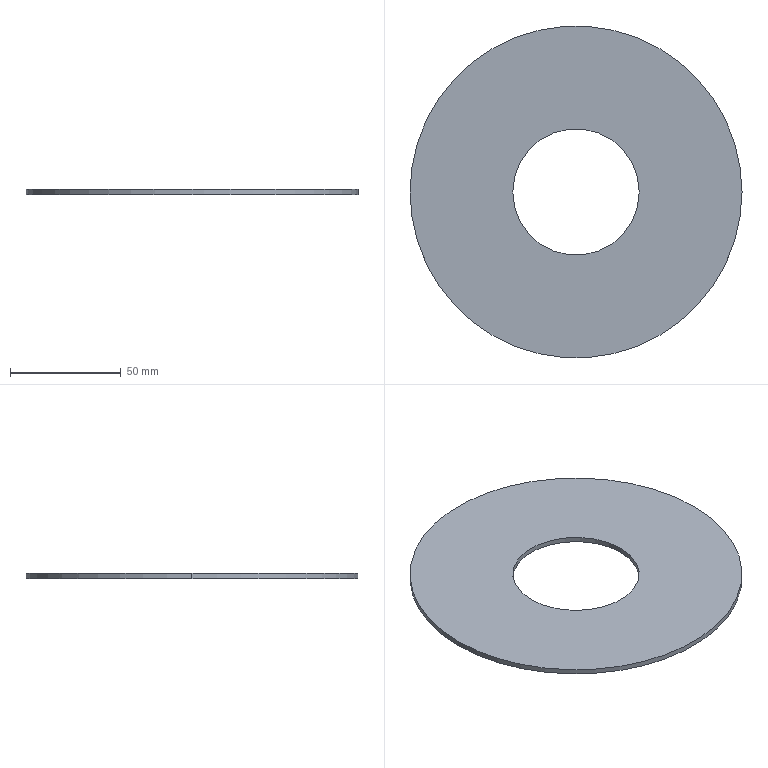Part | SolidWorks | features FlatPattern 1, SMBaseFlange 1, SheetMetal 1 | 1 solid | 6 faces | box 150 x 150 x 2.3 mm | volume 34755 mm3 | cylinder 4 | plane 2 | commonest cylinder face diameters 57.1 x2 150 x2
STEP:
#1=CARTESIAN_POINT('',(-28.55,0.,-2.3));
#2=VERTEX_POINT('',#1);
#3=CARTESIAN_POINT('',(28.55,0.,-2.3));
#4=VERTEX_POINT('',#3);
#5=CARTESIAN_POINT('',(0.,0.,-2.3));
#6=DIRECTION('',(0.,0.,1.));
#7=DIRECTION('',(1.,0.,0.));
#8=AXIS2_PLACEMENT_3D('',#5,#6,#7);
#9=CIRCLE('',#8,28.55);
#10=EDGE_CURVE('',#2,#4,#9,.T.);
#11=ORIENTED_EDGE('',*,*,#10,.F.);
#12=CARTESIAN_POINT('',(-28.55,0.,0.));
#13=VERTEX_POINT('',#12);
#14=CARTESIAN_POINT('',(-28.55,0.,-2.3));
#15=DIRECTION('',(0.,0.,1.));
#16=VECTOR('',#15,1000.);
#17=LINE('',#14,#16);
#18=EDGE_CURVE('',#2,#13,#17,.T.);
#19=ORIENTED_EDGE('',*,*,#18,.T.);
#20=CARTESIAN_POINT('',(28.55,0.,0.));
#21=VERTEX_POINT('',#20);
#22=CARTESIAN_POINT('',(0.,0.,0.));
#23=DIRECTION('',(0.,0.,1.));
#24=DIRECTION('',(1.,0.,0.));
#25=AXIS2_PLACEMENT_3D('',#22,#23,#24);
#26=CIRCLE('',#25,28.55);
#27=EDGE_CURVE('',#13,#21,#26,.T.);
#28=ORIENTED_EDGE('',*,*,#27,.T.);
#29=CARTESIAN_POINT('',(28.55,0.,-2.3));
#30=DIRECTION('',(0.,0.,1.));
#31=VECTOR('',#30,1000.);
#32=LINE('',#29,#31);
#33=EDGE_CURVE('',#4,#21,#32,.T.);
#34=ORIENTED_EDGE('',*,*,#33,.F.);
#35=EDGE_LOOP('',(#11,#19,#28,#34));
#36=FACE_OUTER_BOUND('',#35,.T.);
#37=CARTESIAN_POINT('',(0.,0.,-2.3));
#38=DIRECTION('',(0.,0.,1.));
#39=DIRECTION('',(1.,0.,0.));
#40=AXIS2_PLACEMENT_3D('',#37,#38,#39);
#41=CYLINDRICAL_SURFACE('',#40,28.55);
#42=ADVANCED_FACE('',(#36),#41,.F.);
#43=CARTESIAN_POINT('',(75.,0.,-2.3));
#44=VERTEX_POINT('',#43);
#45=CARTESIAN_POINT('',(-75.,0.,-2.3));
#46=VERTEX_POINT('',#45);
#47=CARTESIAN_POINT('',(0.,0.,-2.3));
#48=DIRECTION('',(0.,0.,1.));
#49=DIRECTION('',(1.,0.,0.));
#50=AXIS2_PLACEMENT_3D('',#47,#48,#49);
#51=CIRCLE('',#50,75.);
#52=EDGE_CURVE('',#44,#46,#51,.T.);
#53=ORIENTED_EDGE('',*,*,#52,.T.);
#54=CARTESIAN_POINT('',(-75.,0.,0.));
#55=VERTEX_POINT('',#54);
#56=CARTESIAN_POINT('',(-75.,0.,-2.3));
#57=DIRECTION('',(0.,0.,1.));
#58=VECTOR('',#57,1000.);
#59=LINE('',#56,#58);
#60=EDGE_CURVE('',#46,#55,#59,.T.);
#61=ORIENTED_EDGE('',*,*,#60,.T.);
#62=CARTESIAN_POINT('',(75.,0.,0.));
#63=VERTEX_POINT('',#62);
#64=CARTESIAN_POINT('',(0.,0.,0.));
#65=DIRECTION('',(0.,0.,1.));
#66=DIRECTION('',(1.,0.,0.));
#67=AXIS2_PLACEMENT_3D('',#64,#65,#66);
#68=CIRCLE('',#67,75.);
#69=EDGE_CURVE('',#63,#55,#68,.T.);
#70=ORIENTED_EDGE('',*,*,#69,.F.);
#71=CARTESIAN_POINT('',(75.,0.,-2.3));
#72=DIRECTION('',(0.,0.,1.));
#73=VECTOR('',#72,1000.);
#74=LINE('',#71,#73);
#75=EDGE_CURVE('',#44,#63,#74,.T.);
#76=ORIENTED_EDGE('',*,*,#75,.F.);
#77=EDGE_LOOP('',(#53,#61,#70,#76));
#78=FACE_OUTER_BOUND('',#77,.T.);
#79=CARTESIAN_POINT('',(0.,0.,-2.3));
#80=DIRECTION('',(0.,0.,1.));
#81=DIRECTION('',(1.,0.,0.));
#82=AXIS2_PLACEMENT_3D('',#79,#80,#81);
#83=CYLINDRICAL_SURFACE('',#82,75.);
#84=ADVANCED_FACE('',(#78),#83,.T.);
#85=ORIENTED_EDGE('',*,*,#60,.F.);
#86=CARTESIAN_POINT('',(0.,0.,-2.3));
#87=DIRECTION('',(0.,0.,1.));
#88=DIRECTION('',(1.,0.,0.));
#89=AXIS2_PLACEMENT_3D('',#86,#87,#88);
#90=CIRCLE('',#89,75.);
#91=EDGE_CURVE('',#46,#44,#90,.T.);
#92=ORIENTED_EDGE('',*,*,#91,.T.);
#93=ORIENTED_EDGE('',*,*,#75,.T.);
#94=CARTESIAN_POINT('',(0.,0.,0.));
#95=DIRECTION('',(0.,0.,1.));
#96=DIRECTION('',(1.,0.,0.));
#97=AXIS2_PLACEMENT_3D('',#94,#95,#96);
#98=CIRCLE('',#97,75.);
#99=EDGE_CURVE('',#55,#63,#98,.T.);
#100=ORIENTED_EDGE('',*,*,#99,.F.);
#101=EDGE_LOOP('',(#85,#92,#93,#100));
#102=FACE_OUTER_BOUND('',#101,.T.);
#103=CARTESIAN_POINT('',(0.,0.,-2.3));
#104=DIRECTION('',(0.,0.,1.));
#105=DIRECTION('',(1.,0.,0.));
#106=AXIS2_PLACEMENT_3D('',#103,#104,#105);
#107=CYLINDRICAL_SURFACE('',#106,75.);
#108=ADVANCED_FACE('',(#102),#107,.T.);
#109=CARTESIAN_POINT('',(0.,0.,-2.3));
#110=DIRECTION('',(0.,0.,1.));
#111=DIRECTION('',(1.,0.,0.));
#112=AXIS2_PLACEMENT_3D('',#109,#110,#111);
#113=CIRCLE('',#112,28.55);
#114=EDGE_CURVE('',#4,#2,#113,.T.);
#115=ORIENTED_EDGE('',*,*,#114,.T.);
#116=ORIENTED_EDGE('',*,*,#10,.T.);
#117=EDGE_LOOP('',(#115,#116));
#118=FACE_BOUND('',#117,.T.);
#119=ORIENTED_EDGE('',*,*,#52,.F.);
#120=ORIENTED_EDGE('',*,*,#91,.F.);
#121=EDGE_LOOP('',(#119,#120));
#122=FACE_OUTER_BOUND('',#121,.T.);
#123=CARTESIAN_POINT('',(0.,0.,-2.3));
#124=DIRECTION('',(0.,0.,1.));
#125=DIRECTION('',(1.,0.,0.));
#126=AXIS2_PLACEMENT_3D('',#123,#124,#125);
#127=PLANE('',#126);
#128=ADVANCED_FACE('',(#118,#122),#127,.F.);
#129=CARTESIAN_POINT('',(0.,0.,0.));
#130=DIRECTION('',(0.,0.,1.));
#131=DIRECTION('',(1.,0.,0.));
#132=AXIS2_PLACEMENT_3D('',#129,#130,#131);
#133=CIRCLE('',#132,28.55);
#134=EDGE_CURVE('',#21,#13,#133,.T.);
#135=ORIENTED_EDGE('',*,*,#134,.F.);
#136=ORIENTED_EDGE('',*,*,#27,.F.);
#137=EDGE_LOOP('',(#135,#136));
#138=FACE_BOUND('',#137,.T.);
#139=ORIENTED_EDGE('',*,*,#69,.T.);
#140=ORIENTED_EDGE('',*,*,#99,.T.);
#141=EDGE_LOOP('',(#139,#140));
#142=FACE_OUTER_BOUND('',#141,.T.);
#143=CARTESIAN_POINT('',(0.,0.,0.));
#144=DIRECTION('',(0.,0.,1.));
#145=DIRECTION('',(1.,0.,0.));
#146=AXIS2_PLACEMENT_3D('',#143,#144,#145);
#147=PLANE('',#146);
#148=ADVANCED_FACE('',(#138,#142),#147,.T.);
#149=ORIENTED_EDGE('',*,*,#18,.F.);
#150=ORIENTED_EDGE('',*,*,#114,.F.);
#151=ORIENTED_EDGE('',*,*,#33,.T.);
#152=ORIENTED_EDGE('',*,*,#134,.T.);
#153=EDGE_LOOP('',(#149,#150,#151,#152));
#154=FACE_OUTER_BOUND('',#153,.T.);
#155=CARTESIAN_POINT('',(0.,0.,-2.3));
#156=DIRECTION('',(0.,0.,1.));
#157=DIRECTION('',(1.,0.,0.));
#158=AXIS2_PLACEMENT_3D('',#155,#156,#157);
#159=CYLINDRICAL_SURFACE('',#158,28.55);
#160=ADVANCED_FACE('',(#154),#159,.F.);
#161=CLOSED_SHELL('',(#42,#84,#108,#128,#148,#160));
#162=MANIFOLD_SOLID_BREP('',#161);
#163=CARTESIAN_POINT('',(0.,0.,0.));
#164=DIRECTION('',(0.,0.,1.));
#165=DIRECTION('',(1.,0.,0.));
#166=AXIS2_PLACEMENT_3D('',#163,#164,#165);
#167=(LENGTH_UNIT()NAMED_UNIT(*)SI_UNIT(.MILLI.,.METRE.));
#168=UNCERTAINTY_MEASURE_WITH_UNIT(LENGTH_MEASURE(0.00001),#167,'','');
#169=(NAMED_UNIT(*)PLANE_ANGLE_UNIT()SI_UNIT($,.RADIAN.));
#170=(NAMED_UNIT(*)SI_UNIT($,.STERADIAN.)SOLID_ANGLE_UNIT());
#171=(GEOMETRIC_REPRESENTATION_CONTEXT(3)GLOBAL_UNCERTAINTY_ASSIGNED_CONTEXT((#168))GLOBAL_UNIT_ASSIGNED_CONTEXT((#167,#169,#170))REPRESENTATION_CONTEXT('',''));
#172=ADVANCED_BREP_SHAPE_REPRESENTATION('',(#162,#166),#171);